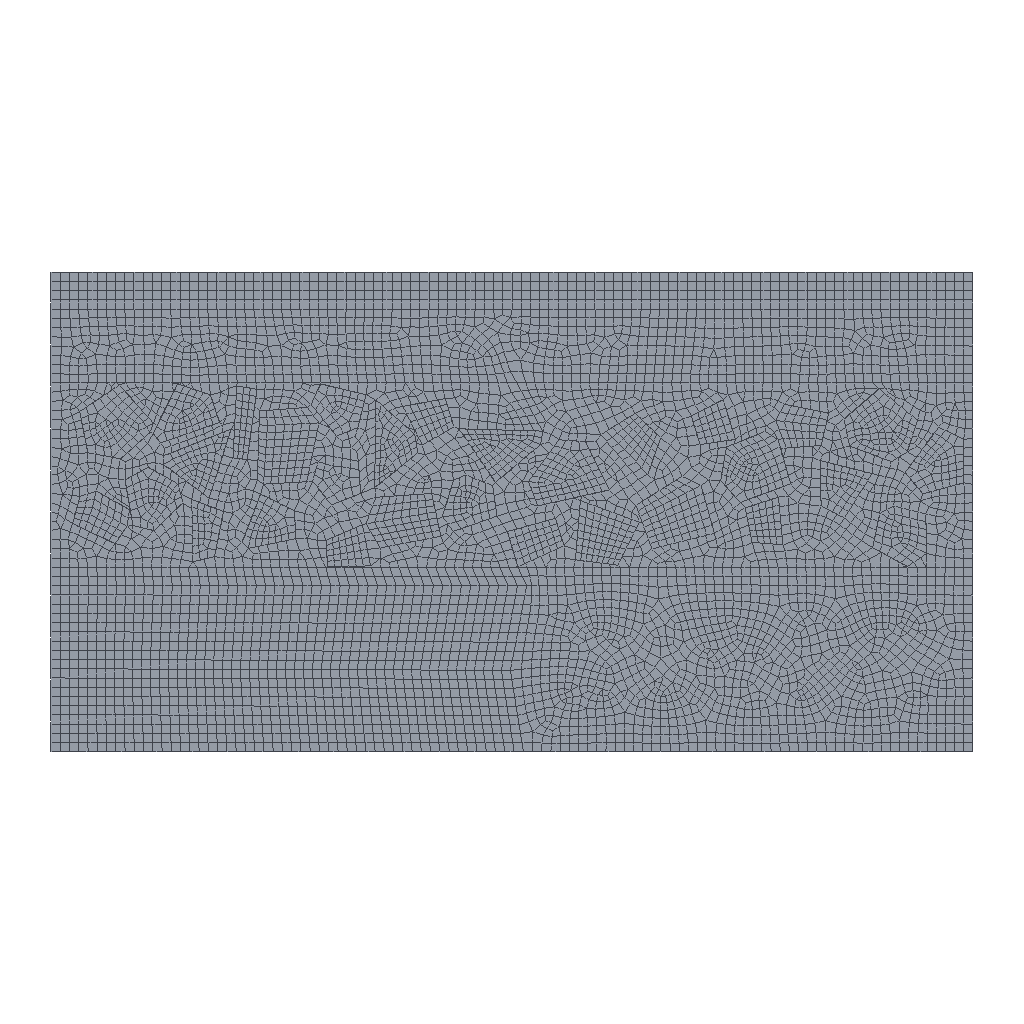Simulation study | abaqus
Set-up summary:
category,name,step,type,value,unit,region
solver,abaqus
solver,version,,,Abaqus/Explicit 2020
units,not stated in the deck,,not stated
analysis,deck,,transient,transient
load_step,Step-1,Step-1,transient,nlgeom=True
contact,interactions,,,general=1 pairs=0 ties=0
load_step,requested,,,1
mesh,nodes,,,7812
mesh,elements,,,7010
element_type,CPS3,,plane,181
element_type,CPS4R,,plane,6175
element_type,COH2D4,,cohesive,654
load,load commands in deck,,count,1
bc,support commands in deck,,count,1
material,COH,,in results
material,COH-2,,in results
material,L1,,in results
material,L2,,in results
material,L4,,in results
material,SHUINI,,in results
material,SUISHI,,in results
check,setup vs results,,match,"per instance, exact: element labels, types and connectivity; labels of the nodes the elements use; coordinates of those nodes at SINGLE_PRECISION in 2 of 2 instance(s)"
Abaqus input file, long lists of numbers shortened:
*Heading
** Job name: Job-1 Model name: Model-1
** Generated by: Abaqus/CAE 2020
*Preprint, echo=NO, model=NO, history=NO, contact=NO
**
** PARTS
**
*Part, name=Part-1
*Node
      1,   512.337,        -520.
      2,    498.249,  -431.699
** (5985 more lines like these left out)
*Element, type=CPS4R
   1, 5318, 5298, 1251,  300
   2, 5298, 5299, 1252, 1251
** (4789 more lines like these left out)
*Element, type=CPS3
1421, 5368, 5369, 5489
1422, 5489, 5369, 5506
** (145 more lines like these left out)
*Element, type=COH2D4
4939, 5298, 5318,    1,  165
4940, 5299, 5298,  165,  166
** (652 more lines like these left out)
*Nset, nset=Set-1
    7,    8,    9,   10,  301,  302,  303,  304,  305,  306,  307,  308,  309,  310,  311,  312
  313,  314,  315,  316,  317,  318,  319,  320,  321,  322,  323,  324,  325,  326,  327,  328
** (30 more lines like these left out)
*Elset, elset=Set-1, generate
 1021,  1420,     1
*Nset, nset=Set-2
    7,    8,   26,   27,   99,  163,  164,  301,  302,  303,  304,  305,  306,  307,  308,  309
  310,  311,  312,  313,  314,  315,  316,  317,  318,  319,  320,  321,  322,  323,  324,  325
** (59 more lines like these left out)
*Elset, elset=Set-2, generate
 4075,  4938,     1
*Nset, nset=Set-3
    4,    5,   26,   27,   98,   99,  182,  183,  184,  185,  186,  187,  188,  189,  190,  191
  192,  193,  194,  195,  196,  197,  198,  199,  200,  201,  202,  203,  204,  205,  206,  207
** (113 more lines like these left out)
*Elset, elset=Set-3, generate
 1421,  2897,     1
*Nset, nset=Set-4
    1,    2,    3,    4,    5,    6,   98,  162,  165,  166,  167,  168,  169,  170,  171,  172
  173,  174,  175,  176,  177,  178,  179,  180,  181,  182,  183,  184,  185,  186,  187,  188
** (144 more lines like these left out)
*Elset, elset=Set-4
    1,    2,    3,    4,    5,    6,    7,    8,    9,   10,   11,   12,   13,   14,   15,   16
   17,   18,   19,   20,   21,   22,   23,   24,   25,   26,   27,   28,   29,   30,   31,   32
** (136 more lines like these left out)
*Nset, nset=Set-5
    1,    2,    3,    4,    5,    6,   98,  162,  165,  166,  167,  168,  169,  170,  171,  172
  173,  174,  175,  176,  177,  178,  179,  180,  181,  182,  183,  184,  185,  186,  187,  188
** (144 more lines like these left out)
*Elset, elset=Set-5
    1,    2,    3,    4,    5,    6,    7,    8,    9,   10,   11,   12,   13,   14,   15,   16
   17,   18,   19,   20,   21,   22,   23,   24,   25,   26,   27,   28,   29,   30,   31,   32
** (136 more lines like these left out)
*Nset, nset=Set-6
    4,    5,   26,   27,   98,   99,  182,  183,  184,  185,  186,  187,  188,  189,  190,  191
  192,  193,  194,  195,  196,  197,  198,  199,  200,  201,  202,  203,  204,  205,  206,  207
** (113 more lines like these left out)
*Elset, elset=Set-6, generate
 1421,  2897,     1
*Elset, elset=CohesiveSeam-1-Elements, generate
 4939,  4987,     1
*Nset, nset=CohesiveSeam-1-TopNodes
    1,    2,    3,    4,   15,   16,   17,   22,   23,   26,  100,  163,  164,  165,  166,  167
  168,  169,  170,  171,  172,  173,  174,  175,  176,  177,  178,  179,  180,  181,  525,  526
** (2 more lines like these left out)
*Nset, nset=CohesiveSeam-1-BottomNodes
   26,  163,  164,  553,  554,  555,  556,  557, 1234, 1235, 1236, 5298, 5299, 5300, 5301, 5302
 5303, 5304, 5305, 5306, 5307, 5308, 5309, 5310, 5311, 5312, 5313, 5314, 5315, 5316, 5317, 5318
** (2 more lines like these left out)
*Nset, nset=CohesiveSeam-1-MidNodes
 164,
*Elset, elset=CohesiveSeam-2-Elements, generate
 4988,  5592,     1
*Nset, nset=CohesiveSeam-2-TopNodes
   11,   12,   13,   14,   15,   16,   18,   19,   20,   21,   24,   25,   28,   29,   30,   31
   32,   33,   34,   35,   36,   37,   38,   39,   40,   41,   42,   43,   44,   45,   46,   47
** (36 more lines like these left out)
*Nset, nset=CohesiveSeam-2-BottomNodes
 5353, 5354, 5355, 5356, 5357, 5358, 5359, 5360, 5361, 5362, 5363, 5364, 5365, 5366, 5367, 5368
 5369, 5370, 5371, 5372, 5373, 5374, 5375, 5377, 5378, 5379, 5380, 5381, 5382, 5383, 5384, 5385
** (36 more lines like these left out)
*Elset, elset=__PickedSurf23_S4, internal
 2192,
*Elset, elset=__PickedSurf23_S3, internal, generate
 4963,  4966,     1
*Surface, type=ELEMENT, name=_PickedSurf23, internal
__PickedSurf23_S4, S4
__PickedSurf23_S3, S3
*Elset, elset=__PickedSurf30_S3, internal
 4974, 4975, 4976, 4977, 4978, 4979, 4980, 4981, 4982, 4983, 4984, 4985, 4986, 4987, 4988, 4989
 4990, 4991, 4992, 4993, 4994, 4995, 4996, 4997, 4998, 4999, 5000, 5001, 5002, 5003, 5004, 5005
** (37 more lines like these left out)
*Surface, type=ELEMENT, name=_PickedSurf30, internal
__PickedSurf30_S3, S3
*Elset, elset=__PickedSurf37_S3, internal
 4939, 4940, 4941, 4942, 4943, 4944, 4945, 4946, 4947, 4948, 4949, 4950, 4951, 4952, 4953, 4954
 4955, 4956, 4957, 4958, 4960, 4961, 4962, 4963, 4964, 4965, 4966, 4968, 4969, 4970, 4971, 4972
** (1 more lines like these left out)
*Elset, elset=__PickedSurf37_S4, internal
 2192, 4180, 4487
*Elset, elset=__PickedSurf37_S1, internal
 4115, 4119, 4967
*Elset, elset=__PickedSurf37_S2, internal
 4118, 4120, 4469, 4488
*Surface, type=ELEMENT, name=_PickedSurf37, internal
__PickedSurf37_S3, S3
__PickedSurf37_S4, S4
__PickedSurf37_S2, S2
__PickedSurf37_S1, S1
*Elset, elset=__PickedSurf44_S3, internal, generate
 4988,  5592,     1
*Surface, type=ELEMENT, name=_PickedSurf44, internal
__PickedSurf44_S3, S3
*Elset, elset=_CohesiveSeam-1-TopSurf_S3, internal, generate
 4939,  4987,     1
*Surface, type=ELEMENT, name=CohesiveSeam-1-TopSurf
_CohesiveSeam-1-TopSurf_S3, S3
*Elset, elset=_CohesiveSeam-1-BottomSurf_S1, internal, generate
 4939,  4987,     1
*Surface, type=ELEMENT, name=CohesiveSeam-1-BottomSurf
_CohesiveSeam-1-BottomSurf_S1, S1
*Elset, elset=_CohesiveSeam-2-TopSurf_S3, internal, generate
 4988,  5592,     1
*Surface, type=ELEMENT, name=CohesiveSeam-2-TopSurf
_CohesiveSeam-2-TopSurf_S3, S3
*Elset, elset=_CohesiveSeam-2-BottomSurf_S1, internal, generate
 4988,  5592,     1
*Surface, type=ELEMENT, name=CohesiveSeam-2-BottomSurf
_CohesiveSeam-2-BottomSurf_S1, S1
** Section: l4
*Solid Section, elset=Set-5, material=l4
,
** Section: l1
*Solid Section, elset=Set-1, material=l1
,
** Section: shuini
*Solid Section, elset=Set-6, material=shuini
,
** Section: l2
*Solid Section, elset=Set-2, material=l2
,
** Section: coh
*Cohesive Section, elset=CohesiveSeam-1-Elements, controls=EC-1, material=coh, response=TRACTION SEPARATION
,
** Section: coh2
*Cohesive Section, elset=CohesiveSeam-2-Elements, controls=EC-1, material=coh-2, response=TRACTION SEPARATION
,
*End Part
**
*Part, name=RVE
*Node
      1,   212.816,   116.648
      2,   223.449,   193.126
** (1823 more lines like these left out)
*Element, type=CPS4R
 1,   1, 148, 789, 169
 2, 148, 149, 790, 789
** (1382 more lines like these left out)
*Element, type=CPS3
542, 1195, 1205, 1208
543, 1202, 1206, 1203
** (32 more lines like these left out)
*Nset, nset=Set-1, generate
    1,  1825,     1
*Elset, elset=Set-1, generate
    1,  1418,     1
** Section: suishi
*Solid Section, elset=Set-1, material=suishi
,
*End Part
**
**
** ASSEMBLY
**
*Assembly, name=Assembly
**
*Instance, name=Part-1-1, part=Part-1
*End Instance
**
*Instance, name=RVE-1, part=RVE
          0.,        -320.,           0.
*End Instance
**
*Nset, nset=Set-1, instance=Part-1-1
    5,    6,   98,  162,  232,  233,  234,  235,  236,  237,  238,  239,  240,  241,  242,  243
  244,  245,  246,  247,  248,  249,  250, 1215, 1216, 1217, 1218, 1219, 1220, 1221, 1222, 1223
** (1 more lines like these left out)
*Elset, elset=Set-1, instance=Part-1-1
 1001, 1002, 1003, 1004, 1005, 1006, 1007, 1008, 1009, 1010, 1011, 1012, 1013, 1014, 1015, 1016
 1017, 1018, 1019, 1020, 3184, 3192, 3193, 3204, 3246, 3266, 3286, 3308, 3309, 3333, 3353, 3400
** (1 more lines like these left out)
*Nset, nset=m_Set-2, instance=RVE-1, generate
    1,  1825,     1
*Elset, elset=m_Set-2, instance=RVE-1, generate
    1,  1418,     1
*Nset, nset=s_Set-2, instance=Part-1-1
    7,    8,    9,   10,   26,   27,   99,  163,  164,  301,  302,  303,  304,  305,  306,  307
  308,  309,  310,  311,  312,  313,  314,  315,  316,  317,  318,  319,  320,  321,  322,  323
** (84 more lines like these left out)
*Elset, elset=s_Set-2, instance=Part-1-1
 1021, 1022, 1023, 1024, 1025, 1026, 1027, 1028, 1029, 1030, 1031, 1032, 1033, 1034, 1035, 1036
 1037, 1038, 1039, 1040, 1041, 1042, 1043, 1044, 1045, 1046, 1047, 1048, 1049, 1050, 1051, 1052
** (77 more lines like these left out)
*Elset, elset=_Surf-1_S3, internal, instance=Part-1-1, generate
 1321,  1420,     1
*Surface, type=ELEMENT, name=Surf-1
_Surf-1_S3, S3
*End Assembly
**
** ELEMENT CONTROLS
**
*Section Controls, name=EC-1, ELEMENT DELETION=YES
1., 1., 1.
**
** MATERIALS
**
*Material, name=coh
*Damage Initiation, criterion=MAXS
5.,5.,5.
*Damage Evolution, type=DISPLACEMENT
 1e-11,
*Density
 2.45e-09,
*Elastic, type=TRACTION
1500.,1500.,1500.
*Material, name=coh-2
*Damage Initiation, criterion=MAXS
6.,6.,6.
*Damage Evolution, type=DISPLACEMENT
 1e-11,
*Density
 3e-09,
*Elastic, type=TRACTION
1000.,1000.,1000.
*Material, name=l1
*Density
 2.3e-09,
*Elastic
1400., 0.35
*Material, name=l2
*Density
 2.2e-09,
*Elastic
1600., 0.35
*Material, name=l4
*Density
 2.45e-09,
*Elastic
1500., 0.3
*Material, name=shuini
*Density
 3e-09,
*Elastic
1000., 0.3
*Material, name=suishi
*Density
 3.5e-09,
*Elastic
15000., 0.2
**
** INTERACTION PROPERTIES
**
*Surface Interaction, name=IntProp-1
*Friction
 0.1,
*Surface Behavior, pressure-overclosure=HARD
** ----------------------------------------------------------------
**
** STEP: Step-1
**
*Step, name=Step-1, nlgeom=YES
*Dynamic, Explicit
, 0.01
*Bulk Viscosity
0.06, 1.2
**
** BOUNDARY CONDITIONS
**
** Name: BC-1 Type: 对称/反对称/完全固定
*Boundary
Set-1, ENCASTRE
**
** LOADS
**
** Name: Load-1   Type: Pressure
*Dsload
Surf-1, P, 7.
**
** INTERACTIONS
**
** Interaction: Int-1
*Contact, op=NEW
*Contact Inclusions, ALL EXTERIOR
*Contact Property Assignment
 ,  , IntProp-1
**
** OUTPUT REQUESTS
**
*Restart, write, number interval=1, time marks=NO
**
** FIELD OUTPUT: F-Output-1
**
*Output, field, number interval=50
*Node Output
A, CF, RF, RM, RT, U, V
*Element Output, directions=YES
E, EVF, LE, MISES, MISESMAX, PE, PEEQ, PEEQVAVG, PEVAVG, S, SDEG, STATUS, SVAVG
*Contact Output
CDISP, CSTRESS
**
** HISTORY OUTPUT: H-Output-1
**
*Output, history, variable=PRESELECT
*End Step
Results summary:
result,step,Step-1,completed,increments=14118 time=0.01/0.01
result,analysis,,,transient
result,last_loadstep,,,1
result,analysis steps,,count,1
result,primary field,,,U
result,reaction total,,FX,481.09,model units
result,reaction total,,FY,8745.107,model units
result,reaction total,,FZ,0.0,model units